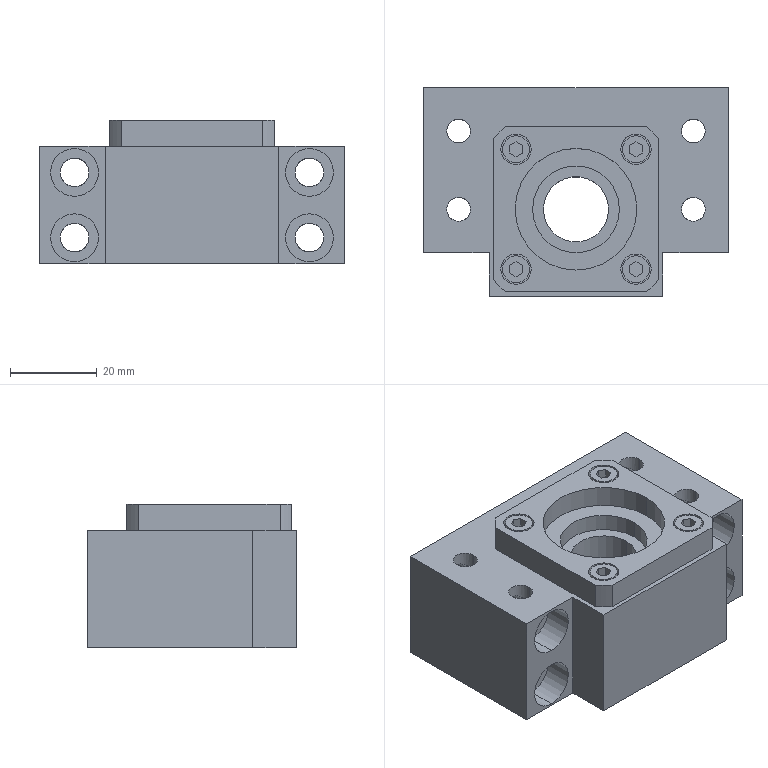Part | SolidWorks | features BaseBody 1 | 1 solid | 129 faces | box 70 x 48 x 33 mm | volume 72753 mm3 | cylinder 70 | plane 59 | commonest cylinder face diameters 5.5 x24 6.2 x8 6.6 x8 7 x8 11 x8 20 x4